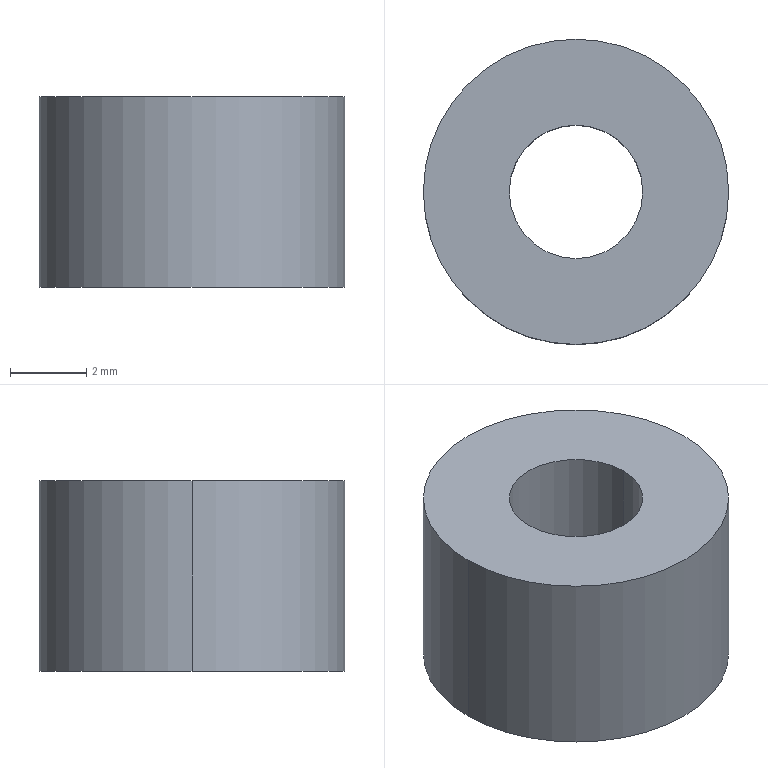Part | SolidWorks | features BaseBody 1 | 1 solid | 6 faces | box 8 x 8 x 5 mm | volume 203.222 mm3 | cylinder 4 | plane 2 | commonest cylinder face diameters 3.5 x2 8 x2
STEP:
#1=CARTESIAN_POINT('',(48.,-49.,0.));
#2=VERTEX_POINT('',#1);
#3=CARTESIAN_POINT('',(40.,-49.,0.));
#4=VERTEX_POINT('',#3);
#5=CARTESIAN_POINT('',(44.,-49.,0.));
#6=DIRECTION('',(0.,0.,1.));
#7=DIRECTION('',(1.,0.,0.));
#8=AXIS2_PLACEMENT_3D('',#5,#6,#7);
#9=CIRCLE('',#8,4.);
#10=EDGE_CURVE('',#2,#4,#9,.T.);
#11=ORIENTED_EDGE('',*,*,#10,.T.);
#12=CARTESIAN_POINT('',(40.,-49.,5.));
#13=VERTEX_POINT('',#12);
#14=CARTESIAN_POINT('',(40.,-49.,0.));
#15=DIRECTION('',(0.,0.,1.));
#16=VECTOR('',#15,1000.);
#17=LINE('',#14,#16);
#18=EDGE_CURVE('',#4,#13,#17,.T.);
#19=ORIENTED_EDGE('',*,*,#18,.T.);
#20=CARTESIAN_POINT('',(48.,-49.,5.));
#21=VERTEX_POINT('',#20);
#22=CARTESIAN_POINT('',(44.,-49.,5.));
#23=DIRECTION('',(0.,0.,-1.));
#24=DIRECTION('',(1.,0.,0.));
#25=AXIS2_PLACEMENT_3D('',#22,#23,#24);
#26=CIRCLE('',#25,4.);
#27=EDGE_CURVE('',#13,#21,#26,.T.);
#28=ORIENTED_EDGE('',*,*,#27,.T.);
#29=CARTESIAN_POINT('',(48.,-49.,0.));
#30=DIRECTION('',(0.,0.,1.));
#31=VECTOR('',#30,1000.);
#32=LINE('',#29,#31);
#33=EDGE_CURVE('',#2,#21,#32,.T.);
#34=ORIENTED_EDGE('',*,*,#33,.F.);
#35=EDGE_LOOP('',(#11,#19,#28,#34));
#36=FACE_OUTER_BOUND('',#35,.T.);
#37=CARTESIAN_POINT('',(44.,-49.,0.));
#38=DIRECTION('',(0.,0.,1.));
#39=DIRECTION('',(1.,0.,0.));
#40=AXIS2_PLACEMENT_3D('',#37,#38,#39);
#41=CYLINDRICAL_SURFACE('',#40,4.);
#42=ADVANCED_FACE('',(#36),#41,.T.);
#43=CARTESIAN_POINT('',(42.25,-49.,0.));
#44=VERTEX_POINT('',#43);
#45=CARTESIAN_POINT('',(45.75,-49.,0.));
#46=VERTEX_POINT('',#45);
#47=CARTESIAN_POINT('',(44.,-49.,0.));
#48=DIRECTION('',(0.,0.,1.));
#49=DIRECTION('',(1.,0.,0.));
#50=AXIS2_PLACEMENT_3D('',#47,#48,#49);
#51=CIRCLE('',#50,1.75);
#52=EDGE_CURVE('',#44,#46,#51,.T.);
#53=ORIENTED_EDGE('',*,*,#52,.F.);
#54=CARTESIAN_POINT('',(42.25,-49.,5.));
#55=VERTEX_POINT('',#54);
#56=CARTESIAN_POINT('',(42.25,-49.,0.));
#57=DIRECTION('',(0.,0.,1.));
#58=VECTOR('',#57,1000.);
#59=LINE('',#56,#58);
#60=EDGE_CURVE('',#44,#55,#59,.T.);
#61=ORIENTED_EDGE('',*,*,#60,.T.);
#62=CARTESIAN_POINT('',(45.75,-49.,5.));
#63=VERTEX_POINT('',#62);
#64=CARTESIAN_POINT('',(44.,-49.,5.));
#65=DIRECTION('',(0.,0.,1.));
#66=DIRECTION('',(1.,0.,0.));
#67=AXIS2_PLACEMENT_3D('',#64,#65,#66);
#68=CIRCLE('',#67,1.75);
#69=EDGE_CURVE('',#55,#63,#68,.T.);
#70=ORIENTED_EDGE('',*,*,#69,.T.);
#71=CARTESIAN_POINT('',(45.75,-49.,0.));
#72=DIRECTION('',(0.,0.,1.));
#73=VECTOR('',#72,1000.);
#74=LINE('',#71,#73);
#75=EDGE_CURVE('',#46,#63,#74,.T.);
#76=ORIENTED_EDGE('',*,*,#75,.F.);
#77=EDGE_LOOP('',(#53,#61,#70,#76));
#78=FACE_OUTER_BOUND('',#77,.T.);
#79=CARTESIAN_POINT('',(44.,-49.,0.));
#80=DIRECTION('',(0.,0.,1.));
#81=DIRECTION('',(1.,0.,0.));
#82=AXIS2_PLACEMENT_3D('',#79,#80,#81);
#83=CYLINDRICAL_SURFACE('',#82,1.75);
#84=ADVANCED_FACE('',(#78),#83,.F.);
#85=ORIENTED_EDGE('',*,*,#18,.F.);
#86=CARTESIAN_POINT('',(44.,-49.,0.));
#87=DIRECTION('',(0.,0.,1.));
#88=DIRECTION('',(1.,0.,0.));
#89=AXIS2_PLACEMENT_3D('',#86,#87,#88);
#90=CIRCLE('',#89,4.);
#91=EDGE_CURVE('',#4,#2,#90,.T.);
#92=ORIENTED_EDGE('',*,*,#91,.T.);
#93=ORIENTED_EDGE('',*,*,#33,.T.);
#94=CARTESIAN_POINT('',(44.,-49.,5.));
#95=DIRECTION('',(0.,0.,-1.));
#96=DIRECTION('',(1.,0.,0.));
#97=AXIS2_PLACEMENT_3D('',#94,#95,#96);
#98=CIRCLE('',#97,4.);
#99=EDGE_CURVE('',#21,#13,#98,.T.);
#100=ORIENTED_EDGE('',*,*,#99,.T.);
#101=EDGE_LOOP('',(#85,#92,#93,#100));
#102=FACE_OUTER_BOUND('',#101,.T.);
#103=CARTESIAN_POINT('',(44.,-49.,0.));
#104=DIRECTION('',(0.,0.,1.));
#105=DIRECTION('',(1.,0.,0.));
#106=AXIS2_PLACEMENT_3D('',#103,#104,#105);
#107=CYLINDRICAL_SURFACE('',#106,4.);
#108=ADVANCED_FACE('',(#102),#107,.T.);
#109=CARTESIAN_POINT('',(44.,-49.,0.));
#110=DIRECTION('',(0.,0.,1.));
#111=DIRECTION('',(1.,0.,0.));
#112=AXIS2_PLACEMENT_3D('',#109,#110,#111);
#113=CIRCLE('',#112,1.75);
#114=EDGE_CURVE('',#46,#44,#113,.T.);
#115=ORIENTED_EDGE('',*,*,#114,.T.);
#116=ORIENTED_EDGE('',*,*,#52,.T.);
#117=EDGE_LOOP('',(#115,#116));
#118=FACE_BOUND('',#117,.T.);
#119=ORIENTED_EDGE('',*,*,#10,.F.);
#120=ORIENTED_EDGE('',*,*,#91,.F.);
#121=EDGE_LOOP('',(#119,#120));
#122=FACE_OUTER_BOUND('',#121,.T.);
#123=CARTESIAN_POINT('',(44.,-49.,0.));
#124=DIRECTION('',(0.,0.,-1.));
#125=DIRECTION('',(-1.,0.,0.));
#126=AXIS2_PLACEMENT_3D('',#123,#124,#125);
#127=PLANE('',#126);
#128=ADVANCED_FACE('',(#118,#122),#127,.T.);
#129=CARTESIAN_POINT('',(44.,-49.,5.));
#130=DIRECTION('',(0.,0.,1.));
#131=DIRECTION('',(1.,0.,0.));
#132=AXIS2_PLACEMENT_3D('',#129,#130,#131);
#133=CIRCLE('',#132,1.75);
#134=EDGE_CURVE('',#63,#55,#133,.T.);
#135=ORIENTED_EDGE('',*,*,#134,.F.);
#136=ORIENTED_EDGE('',*,*,#69,.F.);
#137=EDGE_LOOP('',(#135,#136));
#138=FACE_BOUND('',#137,.T.);
#139=ORIENTED_EDGE('',*,*,#99,.F.);
#140=ORIENTED_EDGE('',*,*,#27,.F.);
#141=EDGE_LOOP('',(#139,#140));
#142=FACE_OUTER_BOUND('',#141,.T.);
#143=CARTESIAN_POINT('',(44.,-49.,5.));
#144=DIRECTION('',(0.,0.,-1.));
#145=DIRECTION('',(-1.,0.,0.));
#146=AXIS2_PLACEMENT_3D('',#143,#144,#145);
#147=PLANE('',#146);
#148=ADVANCED_FACE('',(#138,#142),#147,.F.);
#149=ORIENTED_EDGE('',*,*,#60,.F.);
#150=ORIENTED_EDGE('',*,*,#114,.F.);
#151=ORIENTED_EDGE('',*,*,#75,.T.);
#152=ORIENTED_EDGE('',*,*,#134,.T.);
#153=EDGE_LOOP('',(#149,#150,#151,#152));
#154=FACE_OUTER_BOUND('',#153,.T.);
#155=CARTESIAN_POINT('',(44.,-49.,0.));
#156=DIRECTION('',(0.,0.,1.));
#157=DIRECTION('',(1.,0.,0.));
#158=AXIS2_PLACEMENT_3D('',#155,#156,#157);
#159=CYLINDRICAL_SURFACE('',#158,1.75);
#160=ADVANCED_FACE('',(#154),#159,.F.);
#161=CLOSED_SHELL('',(#42,#84,#108,#128,#148,#160));
#162=MANIFOLD_SOLID_BREP('',#161);
#163=CARTESIAN_POINT('',(0.,0.,0.));
#164=DIRECTION('',(0.,0.,1.));
#165=DIRECTION('',(1.,0.,0.));
#166=AXIS2_PLACEMENT_3D('',#163,#164,#165);
#167=(LENGTH_UNIT()NAMED_UNIT(*)SI_UNIT(.MILLI.,.METRE.));
#168=UNCERTAINTY_MEASURE_WITH_UNIT(LENGTH_MEASURE(0.00001),#167,'','');
#169=(NAMED_UNIT(*)PLANE_ANGLE_UNIT()SI_UNIT($,.RADIAN.));
#170=(NAMED_UNIT(*)SI_UNIT($,.STERADIAN.)SOLID_ANGLE_UNIT());
#171=(GEOMETRIC_REPRESENTATION_CONTEXT(3)GLOBAL_UNCERTAINTY_ASSIGNED_CONTEXT((#168))GLOBAL_UNIT_ASSIGNED_CONTEXT((#167,#169,#170))REPRESENTATION_CONTEXT('',''));
#172=ADVANCED_BREP_SHAPE_REPRESENTATION('',(#162,#166),#171);